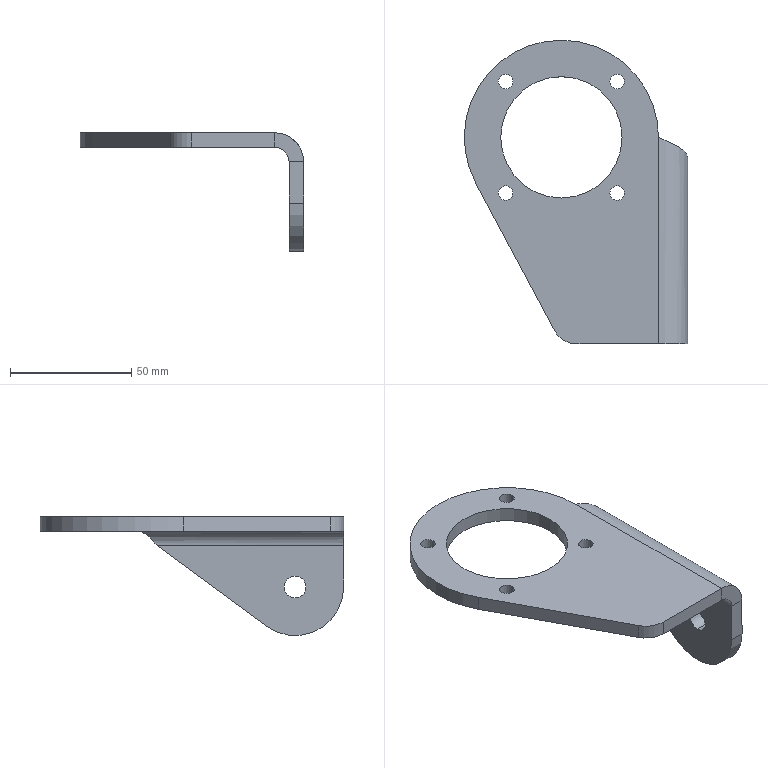Part | STEP file | Microwave Drying Flat Conveyor-CN2500x400-102-102 | 1 solid | 27 faces | box 92 x 125 x 49 mm | volume 51756 mm3 | cylinder 17 | plane 9 | spline 1 | commonest cylinder face diameters 6 x8 9 x2 50 x2 12 x1 20 x1 24 x1
STEP:
#1=CARTESIAN_POINT('',(52.,20.,-33.5));
#2=VERTEX_POINT('',#1);
#3=CARTESIAN_POINT('',(52.,20.,-24.5));
#4=VERTEX_POINT('',#3);
#5=CARTESIAN_POINT('',(52.,20.,-29.));
#6=DIRECTION('',(-1.,0.,0.));
#7=DIRECTION('',(0.,0.,1.));
#8=AXIS2_PLACEMENT_3D('',#5,#6,#7);
#9=CIRCLE('',#8,4.5);
#10=EDGE_CURVE('',#2,#4,#9,.T.);
#11=ORIENTED_EDGE('',*,*,#10,.F.);
#12=CARTESIAN_POINT('',(46.,20.,-33.5));
#13=VERTEX_POINT('',#12);
#14=CARTESIAN_POINT('',(46.,20.,-33.5));
#15=DIRECTION('',(-1.,0.,0.));
#16=VECTOR('',#15,1000.);
#17=LINE('',#14,#16);
#18=EDGE_CURVE('',#2,#13,#17,.T.);
#19=ORIENTED_EDGE('',*,*,#18,.T.);
#20=CARTESIAN_POINT('',(46.,20.,-24.5));
#21=VERTEX_POINT('',#20);
#22=CARTESIAN_POINT('',(46.,20.,-29.));
#23=DIRECTION('',(-1.,0.,0.));
#24=DIRECTION('',(0.,0.,1.));
#25=AXIS2_PLACEMENT_3D('',#22,#23,#24);
#26=CIRCLE('',#25,4.5);
#27=EDGE_CURVE('',#13,#21,#26,.T.);
#28=ORIENTED_EDGE('',*,*,#27,.T.);
#29=CARTESIAN_POINT('',(46.,20.,-24.5));
#30=DIRECTION('',(-1.,0.,0.));
#31=VECTOR('',#30,1000.);
#32=LINE('',#29,#31);
#33=EDGE_CURVE('',#4,#21,#32,.T.);
#34=ORIENTED_EDGE('',*,*,#33,.F.);
#35=EDGE_LOOP('',(#11,#19,#28,#34));
#36=FACE_OUTER_BOUND('',#35,.T.);
#37=CARTESIAN_POINT('',(46.,20.,-29.));
#38=DIRECTION('',(-1.,0.,0.));
#39=DIRECTION('',(0.,0.,1.));
#40=AXIS2_PLACEMENT_3D('',#37,#38,#39);
#41=CYLINDRICAL_SURFACE('',#40,4.5);
#42=ADVANCED_FACE('',(#36),#41,.F.);
#43=CARTESIAN_POINT('',(-25.981,107.981,-6.));
#44=VERTEX_POINT('',#43);
#45=CARTESIAN_POINT('',(-19.981,107.981,-6.));
#46=VERTEX_POINT('',#45);
#47=CARTESIAN_POINT('',(-22.981,107.981,-6.));
#48=DIRECTION('',(0.,0.,1.));
#49=DIRECTION('',(1.,0.,0.));
#50=AXIS2_PLACEMENT_3D('',#47,#48,#49);
#51=CIRCLE('',#50,3.);
#52=EDGE_CURVE('',#44,#46,#51,.T.);
#53=ORIENTED_EDGE('',*,*,#52,.F.);
#54=CARTESIAN_POINT('',(-25.981,107.981,0.));
#55=VERTEX_POINT('',#54);
#56=CARTESIAN_POINT('',(-25.981,107.981,-6.));
#57=DIRECTION('',(0.,0.,1.));
#58=VECTOR('',#57,1000.);
#59=LINE('',#56,#58);
#60=EDGE_CURVE('',#44,#55,#59,.T.);
#61=ORIENTED_EDGE('',*,*,#60,.T.);
#62=CARTESIAN_POINT('',(-19.981,107.981,0.));
#63=VERTEX_POINT('',#62);
#64=CARTESIAN_POINT('',(-22.981,107.981,0.));
#65=DIRECTION('',(0.,0.,1.));
#66=DIRECTION('',(1.,0.,0.));
#67=AXIS2_PLACEMENT_3D('',#64,#65,#66);
#68=CIRCLE('',#67,3.);
#69=EDGE_CURVE('',#55,#63,#68,.T.);
#70=ORIENTED_EDGE('',*,*,#69,.T.);
#71=CARTESIAN_POINT('',(-19.981,107.981,-6.));
#72=DIRECTION('',(0.,0.,1.));
#73=VECTOR('',#72,1000.);
#74=LINE('',#71,#73);
#75=EDGE_CURVE('',#46,#63,#74,.T.);
#76=ORIENTED_EDGE('',*,*,#75,.F.);
#77=EDGE_LOOP('',(#53,#61,#70,#76));
#78=FACE_OUTER_BOUND('',#77,.T.);
#79=CARTESIAN_POINT('',(-22.981,107.981,-6.));
#80=DIRECTION('',(0.,0.,1.));
#81=DIRECTION('',(1.,0.,0.));
#82=AXIS2_PLACEMENT_3D('',#79,#80,#81);
#83=CYLINDRICAL_SURFACE('',#82,3.);
#84=ADVANCED_FACE('',(#78),#83,.F.);
#85=CARTESIAN_POINT('',(-25.981,62.019,-6.));
#86=VERTEX_POINT('',#85);
#87=CARTESIAN_POINT('',(-19.981,62.019,-6.));
#88=VERTEX_POINT('',#87);
#89=CARTESIAN_POINT('',(-22.981,62.019,-6.));
#90=DIRECTION('',(0.,0.,1.));
#91=DIRECTION('',(1.,0.,0.));
#92=AXIS2_PLACEMENT_3D('',#89,#90,#91);
#93=CIRCLE('',#92,3.);
#94=EDGE_CURVE('',#86,#88,#93,.T.);
#95=ORIENTED_EDGE('',*,*,#94,.F.);
#96=CARTESIAN_POINT('',(-25.981,62.019,0.));
#97=VERTEX_POINT('',#96);
#98=CARTESIAN_POINT('',(-25.981,62.019,-6.));
#99=DIRECTION('',(0.,0.,1.));
#100=VECTOR('',#99,1000.);
#101=LINE('',#98,#100);
#102=EDGE_CURVE('',#86,#97,#101,.T.);
#103=ORIENTED_EDGE('',*,*,#102,.T.);
#104=CARTESIAN_POINT('',(-19.981,62.019,0.));
#105=VERTEX_POINT('',#104);
#106=CARTESIAN_POINT('',(-22.981,62.019,0.));
#107=DIRECTION('',(0.,0.,1.));
#108=DIRECTION('',(1.,0.,0.));
#109=AXIS2_PLACEMENT_3D('',#106,#107,#108);
#110=CIRCLE('',#109,3.);
#111=EDGE_CURVE('',#97,#105,#110,.T.);
#112=ORIENTED_EDGE('',*,*,#111,.T.);
#113=CARTESIAN_POINT('',(-19.981,62.019,-6.));
#114=DIRECTION('',(0.,0.,1.));
#115=VECTOR('',#114,1000.);
#116=LINE('',#113,#115);
#117=EDGE_CURVE('',#88,#105,#116,.T.);
#118=ORIENTED_EDGE('',*,*,#117,.F.);
#119=EDGE_LOOP('',(#95,#103,#112,#118));
#120=FACE_OUTER_BOUND('',#119,.T.);
#121=CARTESIAN_POINT('',(-22.981,62.019,-6.));
#122=DIRECTION('',(0.,0.,1.));
#123=DIRECTION('',(1.,0.,0.));
#124=AXIS2_PLACEMENT_3D('',#121,#122,#123);
#125=CYLINDRICAL_SURFACE('',#124,3.);
#126=ADVANCED_FACE('',(#120),#125,.F.);
#127=CARTESIAN_POINT('',(19.981,62.019,-6.));
#128=VERTEX_POINT('',#127);
#129=CARTESIAN_POINT('',(25.981,62.019,-6.));
#130=VERTEX_POINT('',#129);
#131=CARTESIAN_POINT('',(22.981,62.019,-6.));
#132=DIRECTION('',(0.,0.,1.));
#133=DIRECTION('',(1.,0.,0.));
#134=AXIS2_PLACEMENT_3D('',#131,#132,#133);
#135=CIRCLE('',#134,3.);
#136=EDGE_CURVE('',#128,#130,#135,.T.);
#137=ORIENTED_EDGE('',*,*,#136,.F.);
#138=CARTESIAN_POINT('',(19.981,62.019,0.));
#139=VERTEX_POINT('',#138);
#140=CARTESIAN_POINT('',(19.981,62.019,-6.));
#141=DIRECTION('',(0.,0.,1.));
#142=VECTOR('',#141,1000.);
#143=LINE('',#140,#142);
#144=EDGE_CURVE('',#128,#139,#143,.T.);
#145=ORIENTED_EDGE('',*,*,#144,.T.);
#146=CARTESIAN_POINT('',(25.981,62.019,0.));
#147=VERTEX_POINT('',#146);
#148=CARTESIAN_POINT('',(22.981,62.019,0.));
#149=DIRECTION('',(0.,0.,1.));
#150=DIRECTION('',(1.,0.,0.));
#151=AXIS2_PLACEMENT_3D('',#148,#149,#150);
#152=CIRCLE('',#151,3.);
#153=EDGE_CURVE('',#139,#147,#152,.T.);
#154=ORIENTED_EDGE('',*,*,#153,.T.);
#155=CARTESIAN_POINT('',(25.981,62.019,-6.));
#156=DIRECTION('',(0.,0.,1.));
#157=VECTOR('',#156,1000.);
#158=LINE('',#155,#157);
#159=EDGE_CURVE('',#130,#147,#158,.T.);
#160=ORIENTED_EDGE('',*,*,#159,.F.);
#161=EDGE_LOOP('',(#137,#145,#154,#160));
#162=FACE_OUTER_BOUND('',#161,.T.);
#163=CARTESIAN_POINT('',(22.981,62.019,-6.));
#164=DIRECTION('',(0.,0.,1.));
#165=DIRECTION('',(1.,0.,0.));
#166=AXIS2_PLACEMENT_3D('',#163,#164,#165);
#167=CYLINDRICAL_SURFACE('',#166,3.);
#168=ADVANCED_FACE('',(#162),#167,.F.);
#169=CARTESIAN_POINT('',(19.981,107.981,-6.));
#170=VERTEX_POINT('',#169);
#171=CARTESIAN_POINT('',(25.981,107.981,-6.));
#172=VERTEX_POINT('',#171);
#173=CARTESIAN_POINT('',(22.981,107.981,-6.));
#174=DIRECTION('',(0.,0.,1.));
#175=DIRECTION('',(1.,0.,0.));
#176=AXIS2_PLACEMENT_3D('',#173,#174,#175);
#177=CIRCLE('',#176,3.);
#178=EDGE_CURVE('',#170,#172,#177,.T.);
#179=ORIENTED_EDGE('',*,*,#178,.F.);
#180=CARTESIAN_POINT('',(19.981,107.981,0.));
#181=VERTEX_POINT('',#180);
#182=CARTESIAN_POINT('',(19.981,107.981,-6.));
#183=DIRECTION('',(0.,0.,1.));
#184=VECTOR('',#183,1000.);
#185=LINE('',#182,#184);
#186=EDGE_CURVE('',#170,#181,#185,.T.);
#187=ORIENTED_EDGE('',*,*,#186,.T.);
#188=CARTESIAN_POINT('',(25.981,107.981,0.));
#189=VERTEX_POINT('',#188);
#190=CARTESIAN_POINT('',(22.981,107.981,0.));
#191=DIRECTION('',(0.,0.,1.));
#192=DIRECTION('',(1.,0.,0.));
#193=AXIS2_PLACEMENT_3D('',#190,#191,#192);
#194=CIRCLE('',#193,3.);
#195=EDGE_CURVE('',#181,#189,#194,.T.);
#196=ORIENTED_EDGE('',*,*,#195,.T.);
#197=CARTESIAN_POINT('',(25.981,107.981,-6.));
#198=DIRECTION('',(0.,0.,1.));
#199=VECTOR('',#198,1000.);
#200=LINE('',#197,#199);
#201=EDGE_CURVE('',#172,#189,#200,.T.);
#202=ORIENTED_EDGE('',*,*,#201,.F.);
#203=EDGE_LOOP('',(#179,#187,#196,#202));
#204=FACE_OUTER_BOUND('',#203,.T.);
#205=CARTESIAN_POINT('',(22.981,107.981,-6.));
#206=DIRECTION('',(0.,0.,1.));
#207=DIRECTION('',(1.,0.,0.));
#208=AXIS2_PLACEMENT_3D('',#205,#206,#207);
#209=CYLINDRICAL_SURFACE('',#208,3.);
#210=ADVANCED_FACE('',(#204),#209,.F.);
#211=CARTESIAN_POINT('',(-25.,85.,-6.));
#212=VERTEX_POINT('',#211);
#213=CARTESIAN_POINT('',(25.,85.,-6.));
#214=VERTEX_POINT('',#213);
#215=CARTESIAN_POINT('',(0.,85.,-6.));
#216=DIRECTION('',(0.,0.,1.));
#217=DIRECTION('',(1.,0.,0.));
#218=AXIS2_PLACEMENT_3D('',#215,#216,#217);
#219=CIRCLE('',#218,25.);
#220=EDGE_CURVE('',#212,#214,#219,.T.);
#221=ORIENTED_EDGE('',*,*,#220,.F.);
#222=CARTESIAN_POINT('',(-25.,85.,0.));
#223=VERTEX_POINT('',#222);
#224=CARTESIAN_POINT('',(-25.,85.,-6.));
#225=DIRECTION('',(0.,0.,1.));
#226=VECTOR('',#225,1000.);
#227=LINE('',#224,#226);
#228=EDGE_CURVE('',#212,#223,#227,.T.);
#229=ORIENTED_EDGE('',*,*,#228,.T.);
#230=CARTESIAN_POINT('',(25.,85.,0.));
#231=VERTEX_POINT('',#230);
#232=CARTESIAN_POINT('',(0.,85.,0.));
#233=DIRECTION('',(0.,0.,1.));
#234=DIRECTION('',(1.,0.,0.));
#235=AXIS2_PLACEMENT_3D('',#232,#233,#234);
#236=CIRCLE('',#235,25.);
#237=EDGE_CURVE('',#223,#231,#236,.T.);
#238=ORIENTED_EDGE('',*,*,#237,.T.);
#239=CARTESIAN_POINT('',(25.,85.,-6.));
#240=DIRECTION('',(0.,0.,1.));
#241=VECTOR('',#240,1000.);
#242=LINE('',#239,#241);
#243=EDGE_CURVE('',#214,#231,#242,.T.);
#244=ORIENTED_EDGE('',*,*,#243,.F.);
#245=EDGE_LOOP('',(#221,#229,#238,#244));
#246=FACE_OUTER_BOUND('',#245,.T.);
#247=CARTESIAN_POINT('',(0.,85.,-6.));
#248=DIRECTION('',(0.,0.,1.));
#249=DIRECTION('',(1.,0.,0.));
#250=AXIS2_PLACEMENT_3D('',#247,#248,#249);
#251=CYLINDRICAL_SURFACE('',#250,25.);
#252=ADVANCED_FACE('',(#246),#251,.F.);
#253=CARTESIAN_POINT('',(40.,85.,0.));
#254=VERTEX_POINT('',#253);
#255=CARTESIAN_POINT('',(-35.294,66.176,0.));
#256=VERTEX_POINT('',#255);
#257=CARTESIAN_POINT('',(0.,85.,0.));
#258=DIRECTION('',(0.,0.,1.));
#259=DIRECTION('',(1.,0.,0.));
#260=AXIS2_PLACEMENT_3D('',#257,#258,#259);
#261=CIRCLE('',#260,40.);
#262=EDGE_CURVE('',#254,#256,#261,.T.);
#263=ORIENTED_EDGE('',*,*,#262,.F.);
#264=CARTESIAN_POINT('',(40.,85.,-6.));
#265=VERTEX_POINT('',#264);
#266=CARTESIAN_POINT('',(40.,85.,-6.));
#267=DIRECTION('',(0.,0.,1.));
#268=VECTOR('',#267,1000.);
#269=LINE('',#266,#268);
#270=EDGE_CURVE('',#265,#254,#269,.T.);
#271=ORIENTED_EDGE('',*,*,#270,.F.);
#272=CARTESIAN_POINT('',(-35.294,66.176,-6.));
#273=VERTEX_POINT('',#272);
#274=CARTESIAN_POINT('',(0.,85.,-6.));
#275=DIRECTION('',(0.,0.,1.));
#276=DIRECTION('',(1.,0.,0.));
#277=AXIS2_PLACEMENT_3D('',#274,#275,#276);
#278=CIRCLE('',#277,40.);
#279=EDGE_CURVE('',#265,#273,#278,.T.);
#280=ORIENTED_EDGE('',*,*,#279,.T.);
#281=CARTESIAN_POINT('',(-35.294,66.176,-6.));
#282=DIRECTION('',(0.,0.,1.));
#283=VECTOR('',#282,1000.);
#284=LINE('',#281,#283);
#285=EDGE_CURVE('',#273,#256,#284,.T.);
#286=ORIENTED_EDGE('',*,*,#285,.T.);
#287=EDGE_LOOP('',(#263,#271,#280,#286));
#288=FACE_OUTER_BOUND('',#287,.T.);
#289=CARTESIAN_POINT('',(0.,85.,-6.));
#290=DIRECTION('',(0.,0.,1.));
#291=DIRECTION('',(1.,0.,0.));
#292=AXIS2_PLACEMENT_3D('',#289,#290,#291);
#293=CYLINDRICAL_SURFACE('',#292,40.);
#294=ADVANCED_FACE('',(#288),#293,.T.);
#295=CARTESIAN_POINT('',(6.,0.,0.));
#296=VERTEX_POINT('',#295);
#297=CARTESIAN_POINT('',(40.,0.,0.));
#298=VERTEX_POINT('',#297);
#299=CARTESIAN_POINT('',(6.,0.,0.));
#300=DIRECTION('',(1.,0.,0.));
#301=VECTOR('',#300,1000.);
#302=LINE('',#299,#301);
#303=EDGE_CURVE('',#296,#298,#302,.T.);
#304=ORIENTED_EDGE('',*,*,#303,.F.);
#305=CARTESIAN_POINT('',(6.,0.,-6.));
#306=VERTEX_POINT('',#305);
#307=CARTESIAN_POINT('',(6.,0.,-6.));
#308=DIRECTION('',(0.,0.,1.));
#309=VECTOR('',#308,1000.);
#310=LINE('',#307,#309);
#311=EDGE_CURVE('',#306,#296,#310,.T.);
#312=ORIENTED_EDGE('',*,*,#311,.F.);
#313=CARTESIAN_POINT('',(40.,0.,-6.));
#314=VERTEX_POINT('',#313);
#315=CARTESIAN_POINT('',(6.,0.,-6.));
#316=DIRECTION('',(1.,0.,0.));
#317=VECTOR('',#316,1000.);
#318=LINE('',#315,#317);
#319=EDGE_CURVE('',#306,#314,#318,.T.);
#320=ORIENTED_EDGE('',*,*,#319,.T.);
#321=CARTESIAN_POINT('',(40.,0.,-6.));
#322=DIRECTION('',(0.,0.,1.));
#323=VECTOR('',#322,1000.);
#324=LINE('',#321,#323);
#325=EDGE_CURVE('',#314,#298,#324,.T.);
#326=ORIENTED_EDGE('',*,*,#325,.T.);
#327=EDGE_LOOP('',(#304,#312,#320,#326));
#328=FACE_OUTER_BOUND('',#327,.T.);
#329=CARTESIAN_POINT('',(6.,0.,-6.));
#330=DIRECTION('',(0.,-1.,0.));
#331=DIRECTION('',(0.,0.,-1.));
#332=AXIS2_PLACEMENT_3D('',#329,#330,#331);
#333=PLANE('',#332);
#334=ADVANCED_FACE('',(#328),#333,.T.);
#335=CARTESIAN_POINT('',(-2.824,5.294,0.));
#336=VERTEX_POINT('',#335);
#337=CARTESIAN_POINT('',(6.,10.,0.));
#338=DIRECTION('',(0.,0.,1.));
#339=DIRECTION('',(-1.,0.,0.));
#340=AXIS2_PLACEMENT_3D('',#337,#338,#339);
#341=CIRCLE('',#340,10.);
#342=EDGE_CURVE('',#336,#296,#341,.T.);
#343=ORIENTED_EDGE('',*,*,#342,.F.);
#344=CARTESIAN_POINT('',(-2.824,5.294,-6.));
#345=VERTEX_POINT('',#344);
#346=CARTESIAN_POINT('',(-2.824,5.294,-6.));
#347=DIRECTION('',(0.,0.,1.));
#348=VECTOR('',#347,1000.);
#349=LINE('',#346,#348);
#350=EDGE_CURVE('',#345,#336,#349,.T.);
#351=ORIENTED_EDGE('',*,*,#350,.F.);
#352=CARTESIAN_POINT('',(6.,10.,-6.));
#353=DIRECTION('',(0.,0.,1.));
#354=DIRECTION('',(-1.,0.,0.));
#355=AXIS2_PLACEMENT_3D('',#352,#353,#354);
#356=CIRCLE('',#355,10.);
#357=EDGE_CURVE('',#345,#306,#356,.T.);
#358=ORIENTED_EDGE('',*,*,#357,.T.);
#359=ORIENTED_EDGE('',*,*,#311,.T.);
#360=EDGE_LOOP('',(#343,#351,#358,#359));
#361=FACE_OUTER_BOUND('',#360,.T.);
#362=CARTESIAN_POINT('',(6.,10.,-6.));
#363=DIRECTION('',(0.,0.,1.));
#364=DIRECTION('',(1.,0.,0.));
#365=AXIS2_PLACEMENT_3D('',#362,#363,#364);
#366=CYLINDRICAL_SURFACE('',#365,10.);
#367=ADVANCED_FACE('',(#361),#366,.T.);
#368=CARTESIAN_POINT('',(-35.294,66.176,0.));
#369=DIRECTION('',(0.4706,-0.8824,0.));
#370=VECTOR('',#369,1000.);
#371=LINE('',#368,#370);
#372=EDGE_CURVE('',#256,#336,#371,.T.);
#373=ORIENTED_EDGE('',*,*,#372,.F.);
#374=ORIENTED_EDGE('',*,*,#285,.F.);
#375=CARTESIAN_POINT('',(-35.294,66.176,-6.));
#376=DIRECTION('',(0.4706,-0.8824,0.));
#377=VECTOR('',#376,1000.);
#378=LINE('',#375,#377);
#379=EDGE_CURVE('',#273,#345,#378,.T.);
#380=ORIENTED_EDGE('',*,*,#379,.T.);
#381=ORIENTED_EDGE('',*,*,#350,.T.);
#382=EDGE_LOOP('',(#373,#374,#380,#381));
#383=FACE_OUTER_BOUND('',#382,.T.);
#384=CARTESIAN_POINT('',(-35.294,66.176,-6.));
#385=DIRECTION('',(-0.8824,-0.4706,0.));
#386=DIRECTION('',(0.4706,-0.8824,0.));
#387=AXIS2_PLACEMENT_3D('',#384,#385,#386);
#388=PLANE('',#387);
#389=ADVANCED_FACE('',(#383),#388,.T.);
#390=CARTESIAN_POINT('',(-22.981,107.981,-6.));
#391=DIRECTION('',(0.,0.,1.));
#392=DIRECTION('',(1.,0.,0.));
#393=AXIS2_PLACEMENT_3D('',#390,#391,#392);
#394=CIRCLE('',#393,3.);
#395=EDGE_CURVE('',#46,#44,#394,.T.);
#396=ORIENTED_EDGE('',*,*,#395,.T.);
#397=ORIENTED_EDGE('',*,*,#52,.T.);
#398=EDGE_LOOP('',(#396,#397));
#399=FACE_BOUND('',#398,.T.);
#400=CARTESIAN_POINT('',(-22.981,62.019,-6.));
#401=DIRECTION('',(0.,0.,1.));
#402=DIRECTION('',(1.,0.,0.));
#403=AXIS2_PLACEMENT_3D('',#400,#401,#402);
#404=CIRCLE('',#403,3.);
#405=EDGE_CURVE('',#88,#86,#404,.T.);
#406=ORIENTED_EDGE('',*,*,#405,.T.);
#407=ORIENTED_EDGE('',*,*,#94,.T.);
#408=EDGE_LOOP('',(#406,#407));
#409=FACE_BOUND('',#408,.T.);
#410=CARTESIAN_POINT('',(22.981,62.019,-6.));
#411=DIRECTION('',(0.,0.,1.));
#412=DIRECTION('',(1.,0.,0.));
#413=AXIS2_PLACEMENT_3D('',#410,#411,#412);
#414=CIRCLE('',#413,3.);
#415=EDGE_CURVE('',#130,#128,#414,.T.);
#416=ORIENTED_EDGE('',*,*,#415,.T.);
#417=ORIENTED_EDGE('',*,*,#136,.T.);
#418=EDGE_LOOP('',(#416,#417));
#419=FACE_BOUND('',#418,.T.);
#420=CARTESIAN_POINT('',(22.981,107.981,-6.));
#421=DIRECTION('',(0.,0.,1.));
#422=DIRECTION('',(1.,0.,0.));
#423=AXIS2_PLACEMENT_3D('',#420,#421,#422);
#424=CIRCLE('',#423,3.);
#425=EDGE_CURVE('',#172,#170,#424,.T.);
#426=ORIENTED_EDGE('',*,*,#425,.T.);
#427=ORIENTED_EDGE('',*,*,#178,.T.);
#428=EDGE_LOOP('',(#426,#427));
#429=FACE_BOUND('',#428,.T.);
#430=CARTESIAN_POINT('',(0.,85.,-6.));
#431=DIRECTION('',(0.,0.,1.));
#432=DIRECTION('',(1.,0.,0.));
#433=AXIS2_PLACEMENT_3D('',#430,#431,#432);
#434=CIRCLE('',#433,25.);
#435=EDGE_CURVE('',#214,#212,#434,.T.);
#436=ORIENTED_EDGE('',*,*,#435,.T.);
#437=ORIENTED_EDGE('',*,*,#220,.T.);
#438=EDGE_LOOP('',(#436,#437));
#439=FACE_BOUND('',#438,.T.);
#440=ORIENTED_EDGE('',*,*,#279,.F.);
#441=CARTESIAN_POINT('',(40.,85.,-6.));
#442=DIRECTION('',(0.,1.,0.));
#443=VECTOR('',#442,1000.);
#444=LINE('',#441,#443);
#445=EDGE_CURVE('',#314,#265,#444,.T.);
#446=ORIENTED_EDGE('',*,*,#445,.F.);
#447=ORIENTED_EDGE('',*,*,#319,.F.);
#448=ORIENTED_EDGE('',*,*,#357,.F.);
#449=ORIENTED_EDGE('',*,*,#379,.F.);
#450=EDGE_LOOP('',(#440,#446,#447,#448,#449));
#451=FACE_OUTER_BOUND('',#450,.T.);
#452=CARTESIAN_POINT('',(0.,85.,-6.));
#453=DIRECTION('',(0.,0.,1.));
#454=DIRECTION('',(1.,0.,0.));
#455=AXIS2_PLACEMENT_3D('',#452,#453,#454);
#456=PLANE('',#455);
#457=ADVANCED_FACE('',(#399,#409,#419,#429,#439,#451),#456,.F.);
#458=CARTESIAN_POINT('',(-22.981,107.981,0.));
#459=DIRECTION('',(0.,0.,1.));
#460=DIRECTION('',(1.,0.,0.));
#461=AXIS2_PLACEMENT_3D('',#458,#459,#460);
#462=CIRCLE('',#461,3.);
#463=EDGE_CURVE('',#63,#55,#462,.T.);
#464=ORIENTED_EDGE('',*,*,#463,.F.);
#465=ORIENTED_EDGE('',*,*,#69,.F.);
#466=EDGE_LOOP('',(#464,#465));
#467=FACE_BOUND('',#466,.T.);
#468=CARTESIAN_POINT('',(-22.981,62.019,0.));
#469=DIRECTION('',(0.,0.,1.));
#470=DIRECTION('',(1.,0.,0.));
#471=AXIS2_PLACEMENT_3D('',#468,#469,#470);
#472=CIRCLE('',#471,3.);
#473=EDGE_CURVE('',#105,#97,#472,.T.);
#474=ORIENTED_EDGE('',*,*,#473,.F.);
#475=ORIENTED_EDGE('',*,*,#111,.F.);
#476=EDGE_LOOP('',(#474,#475));
#477=FACE_BOUND('',#476,.T.);
#478=CARTESIAN_POINT('',(22.981,62.019,0.));
#479=DIRECTION('',(0.,0.,1.));
#480=DIRECTION('',(1.,0.,0.));
#481=AXIS2_PLACEMENT_3D('',#478,#479,#480);
#482=CIRCLE('',#481,3.);
#483=EDGE_CURVE('',#147,#139,#482,.T.);
#484=ORIENTED_EDGE('',*,*,#483,.F.);
#485=ORIENTED_EDGE('',*,*,#153,.F.);
#486=EDGE_LOOP('',(#484,#485));
#487=FACE_BOUND('',#486,.T.);
#488=CARTESIAN_POINT('',(22.981,107.981,0.));
#489=DIRECTION('',(0.,0.,1.));
#490=DIRECTION('',(1.,0.,0.));
#491=AXIS2_PLACEMENT_3D('',#488,#489,#490);
#492=CIRCLE('',#491,3.);
#493=EDGE_CURVE('',#189,#181,#492,.T.);
#494=ORIENTED_EDGE('',*,*,#493,.F.);
#495=ORIENTED_EDGE('',*,*,#195,.F.);
#496=EDGE_LOOP('',(#494,#495));
#497=FACE_BOUND('',#496,.T.);
#498=CARTESIAN_POINT('',(0.,85.,0.));
#499=DIRECTION('',(0.,0.,1.));
#500=DIRECTION('',(1.,0.,0.));
#501=AXIS2_PLACEMENT_3D('',#498,#499,#500);
#502=CIRCLE('',#501,25.);
#503=EDGE_CURVE('',#231,#223,#502,.T.);
#504=ORIENTED_EDGE('',*,*,#503,.F.);
#505=ORIENTED_EDGE('',*,*,#237,.F.);
#506=EDGE_LOOP('',(#504,#505));
#507=FACE_BOUND('',#506,.T.);
#508=ORIENTED_EDGE('',*,*,#262,.T.);
#509=ORIENTED_EDGE('',*,*,#372,.T.);
#510=ORIENTED_EDGE('',*,*,#342,.T.);
#511=ORIENTED_EDGE('',*,*,#303,.T.);
#512=CARTESIAN_POINT('',(40.,85.,0.));
#513=DIRECTION('',(0.,1.,0.));
#514=VECTOR('',#513,1000.);
#515=LINE('',#512,#514);
#516=EDGE_CURVE('',#298,#254,#515,.T.);
#517=ORIENTED_EDGE('',*,*,#516,.T.);
#518=EDGE_LOOP('',(#508,#509,#510,#511,#517));
#519=FACE_OUTER_BOUND('',#518,.T.);
#520=CARTESIAN_POINT('',(0.,85.,0.));
#521=DIRECTION('',(0.,0.,1.));
#522=DIRECTION('',(1.,0.,0.));
#523=AXIS2_PLACEMENT_3D('',#520,#521,#522);
#524=PLANE('',#523);
#525=ADVANCED_FACE('',(#467,#477,#487,#497,#507,#519),#524,.T.);
#526=ORIENTED_EDGE('',*,*,#228,.F.);
#527=ORIENTED_EDGE('',*,*,#435,.F.);
#528=ORIENTED_EDGE('',*,*,#243,.T.);
#529=ORIENTED_EDGE('',*,*,#503,.T.);
#530=EDGE_LOOP('',(#526,#527,#528,#529));
#531=FACE_OUTER_BOUND('',#530,.T.);
#532=CARTESIAN_POINT('',(0.,85.,-6.));
#533=DIRECTION('',(0.,0.,1.));
#534=DIRECTION('',(1.,0.,0.));
#535=AXIS2_PLACEMENT_3D('',#532,#533,#534);
#536=CYLINDRICAL_SURFACE('',#535,25.);
#537=ADVANCED_FACE('',(#531),#536,.F.);
#538=ORIENTED_EDGE('',*,*,#186,.F.);
#539=ORIENTED_EDGE('',*,*,#425,.F.);
#540=ORIENTED_EDGE('',*,*,#201,.T.);
#541=ORIENTED_EDGE('',*,*,#493,.T.);
#542=EDGE_LOOP('',(#538,#539,#540,#541));
#543=FACE_OUTER_BOUND('',#542,.T.);
#544=CARTESIAN_POINT('',(22.981,107.981,-6.));
#545=DIRECTION('',(0.,0.,1.));
#546=DIRECTION('',(1.,0.,0.));
#547=AXIS2_PLACEMENT_3D('',#544,#545,#546);
#548=CYLINDRICAL_SURFACE('',#547,3.);
#549=ADVANCED_FACE('',(#543),#548,.F.);
#550=ORIENTED_EDGE('',*,*,#144,.F.);
#551=ORIENTED_EDGE('',*,*,#415,.F.);
#552=ORIENTED_EDGE('',*,*,#159,.T.);
#553=ORIENTED_EDGE('',*,*,#483,.T.);
#554=EDGE_LOOP('',(#550,#551,#552,#553));
#555=FACE_OUTER_BOUND('',#554,.T.);
#556=CARTESIAN_POINT('',(22.981,62.019,-6.));
#557=DIRECTION('',(0.,0.,1.));
#558=DIRECTION('',(1.,0.,0.));
#559=AXIS2_PLACEMENT_3D('',#556,#557,#558);
#560=CYLINDRICAL_SURFACE('',#559,3.);
#561=ADVANCED_FACE('',(#555),#560,.F.);
#562=ORIENTED_EDGE('',*,*,#102,.F.);
#563=ORIENTED_EDGE('',*,*,#405,.F.);
#564=ORIENTED_EDGE('',*,*,#117,.T.);
#565=ORIENTED_EDGE('',*,*,#473,.T.);
#566=EDGE_LOOP('',(#562,#563,#564,#565));
#567=FACE_OUTER_BOUND('',#566,.T.);
#568=CARTESIAN_POINT('',(-22.981,62.019,-6.));
#569=DIRECTION('',(0.,0.,1.));
#570=DIRECTION('',(1.,0.,0.));
#571=AXIS2_PLACEMENT_3D('',#568,#569,#570);
#572=CYLINDRICAL_SURFACE('',#571,3.);
#573=ADVANCED_FACE('',(#567),#572,.F.);
#574=ORIENTED_EDGE('',*,*,#60,.F.);
#575=ORIENTED_EDGE('',*,*,#395,.F.);
#576=ORIENTED_EDGE('',*,*,#75,.T.);
#577=ORIENTED_EDGE('',*,*,#463,.T.);
#578=EDGE_LOOP('',(#574,#575,#576,#577));
#579=FACE_OUTER_BOUND('',#578,.T.);
#580=CARTESIAN_POINT('',(-22.981,107.981,-6.));
#581=DIRECTION('',(0.,0.,1.));
#582=DIRECTION('',(1.,0.,0.));
#583=AXIS2_PLACEMENT_3D('',#580,#581,#582);
#584=CYLINDRICAL_SURFACE('',#583,3.);
#585=ADVANCED_FACE('',(#579),#584,.F.);
#586=CARTESIAN_POINT('',(46.,76.846,-12.));
#587=VERTEX_POINT('',#586);
#588=CARTESIAN_POINT('',(52.,76.846,-12.));
#589=VERTEX_POINT('',#588);
#590=CARTESIAN_POINT('',(52.,76.846,-12.));
#591=DIRECTION('',(1.,0.,0.));
#592=VECTOR('',#591,1000.);
#593=LINE('',#590,#592);
#594=EDGE_CURVE('',#587,#589,#593,.T.);
#595=ORIENTED_EDGE('',*,*,#594,.F.);
#596=CARTESIAN_POINT('',(40.,85.,-6.));
#597=CARTESIAN_POINT('',(40.396,84.658,-6.));
#598=CARTESIAN_POINT('',(40.787,84.319,-6.039));
#599=CARTESIAN_POINT('',(41.556,83.641,-6.192));
#600=CARTESIAN_POINT('',(41.933,83.301,-6.306));
#601=CARTESIAN_POINT('',(43.029,82.275,-6.761));
#602=CARTESIAN_POINT('',(43.683,81.608,-7.198));
#603=CARTESIAN_POINT('',(44.379,80.756,-7.894));
#604=CARTESIAN_POINT('',(44.513,80.584,-8.041));
#605=CARTESIAN_POINT('',(44.762,80.244,-8.345));
#606=CARTESIAN_POINT('',(44.879,80.075,-8.503));
#607=CARTESIAN_POINT('',(45.205,79.568,-8.99));
#608=CARTESIAN_POINT('',(45.39,79.231,-9.335));
#609=CARTESIAN_POINT('',(45.691,78.553,-10.058));
#610=CARTESIAN_POINT('',(45.807,78.21,-10.44));
#611=CARTESIAN_POINT('',(45.961,77.528,-11.212));
#612=CARTESIAN_POINT('',(46.,77.189,-11.604));
#613=CARTESIAN_POINT('',(46.,76.846,-12.));
#614=B_SPLINE_CURVE_WITH_KNOTS('',3,(#596,#597,#598,#599,#600,#601,#602,#603,#604,#605,#606,#607,#608,#609,#610,#611,#612,#613),.UNSPECIFIED.,.F.,.F.,(4,2,2,2,2,2,2,2,4),(0.,0.001554,0.003107,0.006215,0.006992,0.007769,0.009322,0.01088,0.01243),.UNSPECIFIED.);
#615=EDGE_CURVE('',#265,#587,#614,.T.);
#616=ORIENTED_EDGE('',*,*,#615,.F.);
#617=ORIENTED_EDGE('',*,*,#270,.T.);
#618=CARTESIAN_POINT('',(40.,85.,0.));
#619=CARTESIAN_POINT('',(40.792,84.657,0.));
#620=CARTESIAN_POINT('',(41.573,84.32,-0.07789));
#621=CARTESIAN_POINT('',(42.722,83.813,-0.3063));
#622=CARTESIAN_POINT('',(43.102,83.644,-0.4012));
#623=CARTESIAN_POINT('',(43.853,83.304,-0.6288));
#624=CARTESIAN_POINT('',(44.227,83.133,-0.7622));
#625=CARTESIAN_POINT('',(45.321,82.62,-1.215));
#626=CARTESIAN_POINT('',(46.012,82.283,-1.585));
#627=CARTESIAN_POINT('',(46.987,81.776,-2.236));
#628=CARTESIAN_POINT('',(47.302,81.607,-2.469));
#629=CARTESIAN_POINT('',(47.911,81.266,-2.968));
#630=CARTESIAN_POINT('',(48.206,81.094,-3.235));
#631=CARTESIAN_POINT('',(49.041,80.583,-4.07));
#632=CARTESIAN_POINT('',(49.537,80.247,-4.675));
#633=CARTESIAN_POINT('',(50.19,79.739,-5.65));
#634=CARTESIAN_POINT('',(50.392,79.569,-5.987));
#635=CARTESIAN_POINT('',(50.765,79.228,-6.683));
#636=CARTESIAN_POINT('',(50.935,79.056,-7.042));
#637=CARTESIAN_POINT('',(51.386,78.547,-8.13));
#638=CARTESIAN_POINT('',(51.613,78.21,-8.878));
#639=CARTESIAN_POINT('',(51.921,77.532,-10.415));
#640=CARTESIAN_POINT('',(52.,77.189,-11.208));
#641=CARTESIAN_POINT('',(52.,76.846,-12.));
#642=B_SPLINE_CURVE_WITH_KNOTS('',3,(#618,#619,#620,#621,#622,#623,#624,#625,#626,#627,#628,#629,#630,#631,#632,#633,#634,#635,#636,#637,#638,#639,#640,#641),.UNSPECIFIED.,.F.,.F.,(4,2,2,2,2,2,2,2,2,2,2,4),(0.,0.002554,0.00383,0.005107,0.007661,0.008938,0.01021,0.01277,0.01404,0.01532,0.01788,0.02043),.UNSPECIFIED.);
#643=EDGE_CURVE('',#254,#589,#642,.T.);
#644=ORIENTED_EDGE('',*,*,#643,.T.);
#645=EDGE_LOOP('',(#595,#616,#617,#644));
#646=FACE_OUTER_BOUND('',#645,.T.);
#647=CARTESIAN_POINT('',(40.,85.,0.06));
#648=CARTESIAN_POINT('',(41.579,84.32,0.06));
#649=CARTESIAN_POINT('',(43.157,83.641,-0.2539));
#650=CARTESIAN_POINT('',(46.074,82.282,-1.462));
#651=CARTESIAN_POINT('',(47.411,81.603,-2.356));
#652=CARTESIAN_POINT('',(49.644,80.244,-4.589));
#653=CARTESIAN_POINT('',(50.538,79.564,-5.926));
#654=CARTESIAN_POINT('',(51.746,78.205,-8.843));
#655=CARTESIAN_POINT('',(52.06,77.526,-10.421));
#656=CARTESIAN_POINT('',(52.06,76.846,-12.));
#657=CARTESIAN_POINT('',(40.,85.,0.));
#658=CARTESIAN_POINT('',(41.571,84.32,0.));
#659=CARTESIAN_POINT('',(43.141,83.641,-0.3123));
#660=CARTESIAN_POINT('',(46.043,82.282,-1.515));
#661=CARTESIAN_POINT('',(47.375,81.603,-2.404));
#662=CARTESIAN_POINT('',(49.596,80.244,-4.625));
#663=CARTESIAN_POINT('',(50.485,79.564,-5.957));
#664=CARTESIAN_POINT('',(51.688,78.205,-8.859));
#665=CARTESIAN_POINT('',(52.,77.526,-10.429));
#666=CARTESIAN_POINT('',(52.,76.846,-12.));
#667=CARTESIAN_POINT('',(40.,85.,-6.));
#668=CARTESIAN_POINT('',(40.785,84.32,-6.));
#669=CARTESIAN_POINT('',(41.57,83.641,-6.156));
#670=CARTESIAN_POINT('',(43.022,82.282,-6.757));
#671=CARTESIAN_POINT('',(43.687,81.603,-7.202));
#672=CARTESIAN_POINT('',(44.798,80.244,-8.313));
#673=CARTESIAN_POINT('',(45.243,79.564,-8.978));
#674=CARTESIAN_POINT('',(45.844,78.205,-10.43));
#675=CARTESIAN_POINT('',(46.,77.526,-11.215));
#676=CARTESIAN_POINT('',(46.,76.846,-12.));
#677=CARTESIAN_POINT('',(40.,85.,-6.061));
#678=CARTESIAN_POINT('',(40.778,84.32,-6.061));
#679=CARTESIAN_POINT('',(41.555,83.641,-6.215));
#680=CARTESIAN_POINT('',(42.991,82.282,-6.81));
#681=CARTESIAN_POINT('',(43.65,81.603,-7.25));
#682=CARTESIAN_POINT('',(44.75,80.244,-8.35));
#683=CARTESIAN_POINT('',(45.19,79.564,-9.009));
#684=CARTESIAN_POINT('',(45.785,78.205,-10.445));
#685=CARTESIAN_POINT('',(45.939,77.526,-11.222));
#686=CARTESIAN_POINT('',(45.939,76.846,-12.));
#687=B_SPLINE_SURFACE_WITH_KNOTS('',1,3,((#647,#648,#649,#650,#651,#652,#653,#654,#655,#656),(#657,#658,#659,#660,#661,#662,#663,#664,#665,#666),(#667,#668,#669,#670,#671,#672,#673,#674,#675,#676),(#677,#678,#679,#680,#681,#682,#683,#684,#685,#686)),.UNSPECIFIED.,.F.,.F.,.F.,(2,1,1,2),(4,2,2,2,4),(-0.01,0.,1.,1.01),(0.,0.25,0.5,0.75,1.),.UNSPECIFIED.);
#688=ADVANCED_FACE('',(#646),#687,.F.);
#689=CARTESIAN_POINT('',(46.,0.,-12.));
#690=VERTEX_POINT('',#689);
#691=CARTESIAN_POINT('',(40.,0.,-12.));
#692=DIRECTION('',(0.,-1.,0.));
#693=DIRECTION('',(0.,0.,-1.));
#694=AXIS2_PLACEMENT_3D('',#691,#692,#693);
#695=CIRCLE('',#694,6.);
#696=EDGE_CURVE('',#690,#314,#695,.T.);
#697=ORIENTED_EDGE('',*,*,#696,.F.);
#698=CARTESIAN_POINT('',(52.,0.,-12.));
#699=VERTEX_POINT('',#698);
#700=CARTESIAN_POINT('',(46.,0.,-12.));
#701=DIRECTION('',(1.,0.,0.));
#702=VECTOR('',#701,1000.);
#703=LINE('',#700,#702);
#704=EDGE_CURVE('',#690,#699,#703,.T.);
#705=ORIENTED_EDGE('',*,*,#704,.T.);
#706=CARTESIAN_POINT('',(40.,0.,-12.));
#707=DIRECTION('',(0.,-1.,0.));
#708=DIRECTION('',(0.,0.,-1.));
#709=AXIS2_PLACEMENT_3D('',#706,#707,#708);
#710=CIRCLE('',#709,12.);
#711=EDGE_CURVE('',#699,#298,#710,.T.);
#712=ORIENTED_EDGE('',*,*,#711,.T.);
#713=ORIENTED_EDGE('',*,*,#325,.F.);
#714=EDGE_LOOP('',(#697,#705,#712,#713));
#715=FACE_OUTER_BOUND('',#714,.T.);
#716=CARTESIAN_POINT('',(40.,0.,-12.));
#717=DIRECTION('',(0.,1.,0.));
#718=DIRECTION('',(0.,0.,1.));
#719=AXIS2_PLACEMENT_3D('',#716,#717,#718);
#720=PLANE('',#719);
#721=ADVANCED_FACE('',(#715),#720,.F.);
#722=ORIENTED_EDGE('',*,*,#516,.F.);
#723=ORIENTED_EDGE('',*,*,#711,.F.);
#724=CARTESIAN_POINT('',(52.,76.846,-12.));
#725=DIRECTION('',(0.,1.,0.));
#726=VECTOR('',#725,1000.);
#727=LINE('',#724,#726);
#728=EDGE_CURVE('',#699,#589,#727,.T.);
#729=ORIENTED_EDGE('',*,*,#728,.T.);
#730=ORIENTED_EDGE('',*,*,#643,.F.);
#731=EDGE_LOOP('',(#722,#723,#729,#730));
#732=FACE_OUTER_BOUND('',#731,.T.);
#733=CARTESIAN_POINT('',(40.,0.,-12.));
#734=DIRECTION('',(0.,-1.,0.));
#735=DIRECTION('',(1.,0.,0.));
#736=AXIS2_PLACEMENT_3D('',#733,#734,#735);
#737=CYLINDRICAL_SURFACE('',#736,12.);
#738=ADVANCED_FACE('',(#732),#737,.T.);
#739=ORIENTED_EDGE('',*,*,#445,.T.);
#740=ORIENTED_EDGE('',*,*,#615,.T.);
#741=CARTESIAN_POINT('',(46.,76.846,-12.));
#742=DIRECTION('',(0.,-1.,0.));
#743=VECTOR('',#742,1000.);
#744=LINE('',#741,#743);
#745=EDGE_CURVE('',#587,#690,#744,.T.);
#746=ORIENTED_EDGE('',*,*,#745,.T.);
#747=ORIENTED_EDGE('',*,*,#696,.T.);
#748=EDGE_LOOP('',(#739,#740,#746,#747));
#749=FACE_OUTER_BOUND('',#748,.T.);
#750=CARTESIAN_POINT('',(40.,0.,-12.));
#751=DIRECTION('',(0.,-1.,0.));
#752=DIRECTION('',(1.,0.,0.));
#753=AXIS2_PLACEMENT_3D('',#750,#751,#752);
#754=CYLINDRICAL_SURFACE('',#753,6.);
#755=ADVANCED_FACE('',(#749),#754,.F.);
#756=CARTESIAN_POINT('',(52.,0.,-29.));
#757=VERTEX_POINT('',#756);
#758=CARTESIAN_POINT('',(52.,0.,-6.));
#759=DIRECTION('',(0.,0.,1.));
#760=VECTOR('',#759,1000.);
#761=LINE('',#758,#760);
#762=EDGE_CURVE('',#757,#699,#761,.T.);
#763=ORIENTED_EDGE('',*,*,#762,.T.);
#764=ORIENTED_EDGE('',*,*,#704,.F.);
#765=CARTESIAN_POINT('',(46.,0.,-29.));
#766=VERTEX_POINT('',#765);
#767=CARTESIAN_POINT('',(46.,0.,-29.));
#768=DIRECTION('',(0.,0.,1.));
#769=VECTOR('',#768,1000.);
#770=LINE('',#767,#769);
#771=EDGE_CURVE('',#766,#690,#770,.T.);
#772=ORIENTED_EDGE('',*,*,#771,.F.);
#773=CARTESIAN_POINT('',(52.,0.,-29.));
#774=DIRECTION('',(-1.,0.,0.));
#775=VECTOR('',#774,1000.);
#776=LINE('',#773,#775);
#777=EDGE_CURVE('',#757,#766,#776,.T.);
#778=ORIENTED_EDGE('',*,*,#777,.F.);
#779=EDGE_LOOP('',(#763,#764,#772,#778));
#780=FACE_OUTER_BOUND('',#779,.T.);
#781=CARTESIAN_POINT('',(52.,0.,-6.));
#782=DIRECTION('',(0.,-1.,0.));
#783=DIRECTION('',(0.,0.,-1.));
#784=AXIS2_PLACEMENT_3D('',#781,#782,#783);
#785=PLANE('',#784);
#786=ADVANCED_FACE('',(#780),#785,.T.);
#787=CARTESIAN_POINT('',(46.,31.854,-45.109));
#788=VERTEX_POINT('',#787);
#789=CARTESIAN_POINT('',(46.,31.854,-45.109));
#790=DIRECTION('',(0.,-0.8054,-0.5927));
#791=VECTOR('',#790,1000.);
#792=LINE('',#789,#791);
#793=EDGE_CURVE('',#587,#788,#792,.T.);
#794=ORIENTED_EDGE('',*,*,#793,.F.);
#795=ORIENTED_EDGE('',*,*,#594,.T.);
#796=CARTESIAN_POINT('',(52.,31.854,-45.109));
#797=VERTEX_POINT('',#796);
#798=CARTESIAN_POINT('',(52.,31.854,-45.109));
#799=DIRECTION('',(0.,-0.8054,-0.5927));
#800=VECTOR('',#799,1000.);
#801=LINE('',#798,#800);
#802=EDGE_CURVE('',#589,#797,#801,.T.);
#803=ORIENTED_EDGE('',*,*,#802,.T.);
#804=CARTESIAN_POINT('',(52.,31.854,-45.109));
#805=DIRECTION('',(-1.,0.,0.));
#806=VECTOR('',#805,1000.);
#807=LINE('',#804,#806);
#808=EDGE_CURVE('',#797,#788,#807,.T.);
#809=ORIENTED_EDGE('',*,*,#808,.T.);
#810=EDGE_LOOP('',(#794,#795,#803,#809));
#811=FACE_OUTER_BOUND('',#810,.T.);
#812=CARTESIAN_POINT('',(52.,31.854,-45.109));
#813=DIRECTION('',(0.,0.5927,-0.8054));
#814=DIRECTION('',(0.,0.8054,0.5927));
#815=AXIS2_PLACEMENT_3D('',#812,#813,#814);
#816=PLANE('',#815);
#817=ADVANCED_FACE('',(#811),#816,.T.);
#818=CARTESIAN_POINT('',(52.,20.,-29.));
#819=DIRECTION('',(-1.,0.,0.));
#820=DIRECTION('',(0.,0.,1.));
#821=AXIS2_PLACEMENT_3D('',#818,#819,#820);
#822=CIRCLE('',#821,4.5);
#823=EDGE_CURVE('',#4,#2,#822,.T.);
#824=ORIENTED_EDGE('',*,*,#823,.T.);
#825=ORIENTED_EDGE('',*,*,#10,.T.);
#826=EDGE_LOOP('',(#824,#825));
#827=FACE_BOUND('',#826,.T.);
#828=ORIENTED_EDGE('',*,*,#728,.F.);
#829=ORIENTED_EDGE('',*,*,#762,.F.);
#830=CARTESIAN_POINT('',(52.,20.,-29.));
#831=DIRECTION('',(-1.,0.,0.));
#832=DIRECTION('',(0.,0.,1.));
#833=AXIS2_PLACEMENT_3D('',#830,#831,#832);
#834=CIRCLE('',#833,20.);
#835=EDGE_CURVE('',#797,#757,#834,.T.);
#836=ORIENTED_EDGE('',*,*,#835,.F.);
#837=ORIENTED_EDGE('',*,*,#802,.F.);
#838=EDGE_LOOP('',(#828,#829,#836,#837));
#839=FACE_OUTER_BOUND('',#838,.T.);
#840=CARTESIAN_POINT('',(52.,20.,-29.));
#841=DIRECTION('',(-1.,0.,0.));
#842=DIRECTION('',(0.,0.,1.));
#843=AXIS2_PLACEMENT_3D('',#840,#841,#842);
#844=PLANE('',#843);
#845=ADVANCED_FACE('',(#827,#839),#844,.F.);
#846=CARTESIAN_POINT('',(46.,20.,-29.));
#847=DIRECTION('',(-1.,0.,0.));
#848=DIRECTION('',(0.,0.,1.));
#849=AXIS2_PLACEMENT_3D('',#846,#847,#848);
#850=CIRCLE('',#849,4.5);
#851=EDGE_CURVE('',#21,#13,#850,.T.);
#852=ORIENTED_EDGE('',*,*,#851,.F.);
#853=ORIENTED_EDGE('',*,*,#27,.F.);
#854=EDGE_LOOP('',(#852,#853));
#855=FACE_BOUND('',#854,.T.);
#856=ORIENTED_EDGE('',*,*,#771,.T.);
#857=ORIENTED_EDGE('',*,*,#745,.F.);
#858=ORIENTED_EDGE('',*,*,#793,.T.);
#859=CARTESIAN_POINT('',(46.,20.,-29.));
#860=DIRECTION('',(-1.,0.,0.));
#861=DIRECTION('',(0.,0.,1.));
#862=AXIS2_PLACEMENT_3D('',#859,#860,#861);
#863=CIRCLE('',#862,20.);
#864=EDGE_CURVE('',#788,#766,#863,.T.);
#865=ORIENTED_EDGE('',*,*,#864,.T.);
#866=EDGE_LOOP('',(#856,#857,#858,#865));
#867=FACE_OUTER_BOUND('',#866,.T.);
#868=CARTESIAN_POINT('',(46.,20.,-29.));
#869=DIRECTION('',(-1.,0.,0.));
#870=DIRECTION('',(0.,0.,1.));
#871=AXIS2_PLACEMENT_3D('',#868,#869,#870);
#872=PLANE('',#871);
#873=ADVANCED_FACE('',(#855,#867),#872,.T.);
#874=ORIENTED_EDGE('',*,*,#864,.F.);
#875=ORIENTED_EDGE('',*,*,#808,.F.);
#876=ORIENTED_EDGE('',*,*,#835,.T.);
#877=ORIENTED_EDGE('',*,*,#777,.T.);
#878=EDGE_LOOP('',(#874,#875,#876,#877));
#879=FACE_OUTER_BOUND('',#878,.T.);
#880=CARTESIAN_POINT('',(52.,20.,-29.));
#881=DIRECTION('',(-1.,0.,0.));
#882=DIRECTION('',(0.,0.,1.));
#883=AXIS2_PLACEMENT_3D('',#880,#881,#882);
#884=CYLINDRICAL_SURFACE('',#883,20.);
#885=ADVANCED_FACE('',(#879),#884,.T.);
#886=ORIENTED_EDGE('',*,*,#18,.F.);
#887=ORIENTED_EDGE('',*,*,#823,.F.);
#888=ORIENTED_EDGE('',*,*,#33,.T.);
#889=ORIENTED_EDGE('',*,*,#851,.T.);
#890=EDGE_LOOP('',(#886,#887,#888,#889));
#891=FACE_OUTER_BOUND('',#890,.T.);
#892=CARTESIAN_POINT('',(46.,20.,-29.));
#893=DIRECTION('',(-1.,0.,0.));
#894=DIRECTION('',(0.,0.,1.));
#895=AXIS2_PLACEMENT_3D('',#892,#893,#894);
#896=CYLINDRICAL_SURFACE('',#895,4.5);
#897=ADVANCED_FACE('',(#891),#896,.F.);
#898=CLOSED_SHELL('',(#42,#84,#126,#168,#210,#252,#294,#334,#367,#389,#457,#525,#537,#549,#561,#573,#585,#688,#721,#738,#755,#786,#817,#845,#873,#885,#897));
#899=MANIFOLD_SOLID_BREP('',#898);
#900=CARTESIAN_POINT('',(0.,0.,0.));
#901=DIRECTION('',(0.,0.,1.));
#902=DIRECTION('',(1.,0.,0.));
#903=AXIS2_PLACEMENT_3D('',#900,#901,#902);
#904=(LENGTH_UNIT()NAMED_UNIT(*)SI_UNIT(.MILLI.,.METRE.));
#905=UNCERTAINTY_MEASURE_WITH_UNIT(LENGTH_MEASURE(0.00001),#904,'','');
#906=(NAMED_UNIT(*)PLANE_ANGLE_UNIT()SI_UNIT($,.RADIAN.));
#907=(NAMED_UNIT(*)SI_UNIT($,.STERADIAN.)SOLID_ANGLE_UNIT());
#908=(GEOMETRIC_REPRESENTATION_CONTEXT(3)GLOBAL_UNCERTAINTY_ASSIGNED_CONTEXT((#905))GLOBAL_UNIT_ASSIGNED_CONTEXT((#904,#906,#907))REPRESENTATION_CONTEXT('',''));
#909=ADVANCED_BREP_SHAPE_REPRESENTATION('',(#899,#903),#908);